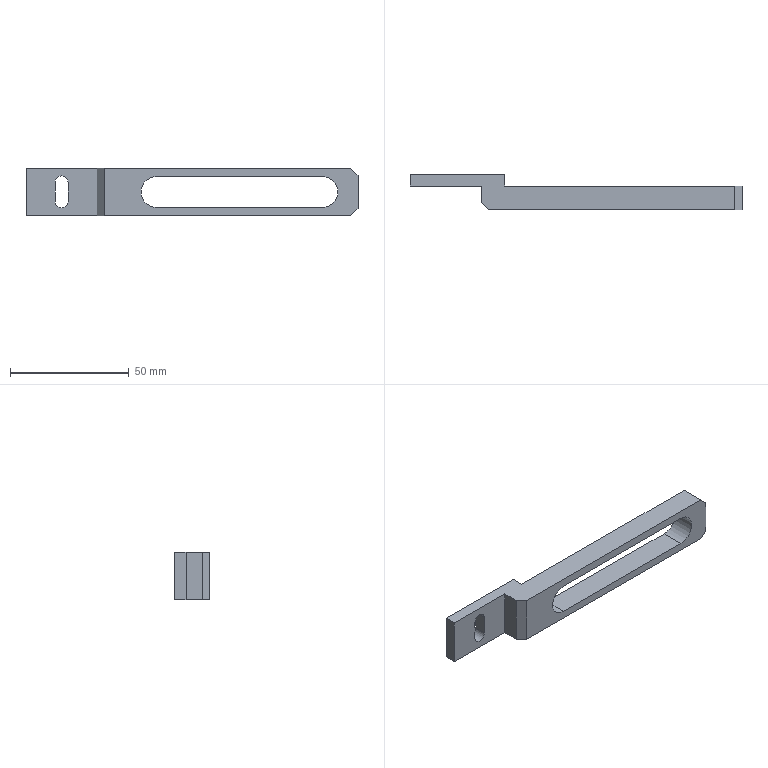Part | SolidWorks | features ICE 3, Chamfer 2, Extrusion 1 | 1 solid | 22 faces | box 140 x 15 x 20 mm | volume 15054 mm3 | plane 17 | cylinder 5 | commonest cylinder face diameters 5.5 x3 13 x2
STEP:
#1=CARTESIAN_POINT('',(15.,-5.,6.75));
#2=VERTEX_POINT('',#1);
#3=CARTESIAN_POINT('',(17.75,-5.,4.));
#4=VERTEX_POINT('',#3);
#5=CARTESIAN_POINT('',(15.,-5.,4.));
#6=DIRECTION('',(0.,1.,0.));
#7=DIRECTION('',(-1.,0.,0.));
#8=AXIS2_PLACEMENT_3D('',#5,#6,#7);
#9=CIRCLE('',#8,2.75);
#10=EDGE_CURVE('',#2,#4,#9,.T.);
#11=ORIENTED_EDGE('',*,*,#10,.F.);
#12=CARTESIAN_POINT('',(15.,0.,6.75));
#13=VERTEX_POINT('',#12);
#14=CARTESIAN_POINT('',(15.,-15.,6.75));
#15=DIRECTION('',(0.,1.,0.));
#16=VECTOR('',#15,1000.);
#17=LINE('',#14,#16);
#18=EDGE_CURVE('',#2,#13,#17,.T.);
#19=ORIENTED_EDGE('',*,*,#18,.T.);
#20=CARTESIAN_POINT('',(17.75,0.,4.));
#21=VERTEX_POINT('',#20);
#22=CARTESIAN_POINT('',(15.,0.,4.));
#23=DIRECTION('',(0.,1.,0.));
#24=DIRECTION('',(0.,0.,1.));
#25=AXIS2_PLACEMENT_3D('',#22,#23,#24);
#26=CIRCLE('',#25,2.75);
#27=EDGE_CURVE('',#13,#21,#26,.T.);
#28=ORIENTED_EDGE('',*,*,#27,.T.);
#29=CARTESIAN_POINT('',(17.75,-15.,4.));
#30=DIRECTION('',(0.,1.,0.));
#31=VECTOR('',#30,1000.);
#32=LINE('',#29,#31);
#33=EDGE_CURVE('',#4,#21,#32,.T.);
#34=ORIENTED_EDGE('',*,*,#33,.F.);
#35=EDGE_LOOP('',(#11,#19,#28,#34));
#36=FACE_OUTER_BOUND('',#35,.T.);
#37=CARTESIAN_POINT('',(15.,-15.,4.));
#38=DIRECTION('',(0.,1.,0.));
#39=DIRECTION('',(0.,0.,1.));
#40=AXIS2_PLACEMENT_3D('',#37,#38,#39);
#41=CYLINDRICAL_SURFACE('',#40,2.75);
#42=ADVANCED_FACE('',(#36),#41,.F.);
#43=CARTESIAN_POINT('',(0.,0.,-10.));
#44=VERTEX_POINT('',#43);
#45=CARTESIAN_POINT('',(0.,-5.,-10.));
#46=VERTEX_POINT('',#45);
#47=CARTESIAN_POINT('',(0.,-5.,-10.));
#48=DIRECTION('',(0.,-1.,0.));
#49=VECTOR('',#48,1000.);
#50=LINE('',#47,#49);
#51=EDGE_CURVE('',#44,#46,#50,.T.);
#52=ORIENTED_EDGE('',*,*,#51,.T.);
#53=CARTESIAN_POINT('',(0.,-5.,10.));
#54=VERTEX_POINT('',#53);
#55=CARTESIAN_POINT('',(0.,-5.,10.));
#56=DIRECTION('',(0.,0.,-1.));
#57=VECTOR('',#56,1000.);
#58=LINE('',#55,#57);
#59=EDGE_CURVE('',#54,#46,#58,.T.);
#60=ORIENTED_EDGE('',*,*,#59,.F.);
#61=CARTESIAN_POINT('',(0.,0.,10.));
#62=VERTEX_POINT('',#61);
#63=CARTESIAN_POINT('',(0.,-5.,10.));
#64=DIRECTION('',(0.,-1.,0.));
#65=VECTOR('',#64,1000.);
#66=LINE('',#63,#65);
#67=EDGE_CURVE('',#62,#54,#66,.T.);
#68=ORIENTED_EDGE('',*,*,#67,.F.);
#69=CARTESIAN_POINT('',(0.,0.,10.));
#70=DIRECTION('',(0.,0.,-1.));
#71=VECTOR('',#70,1000.);
#72=LINE('',#69,#71);
#73=EDGE_CURVE('',#62,#44,#72,.T.);
#74=ORIENTED_EDGE('',*,*,#73,.T.);
#75=EDGE_LOOP('',(#52,#60,#68,#74));
#76=FACE_OUTER_BOUND('',#75,.T.);
#77=CARTESIAN_POINT('',(0.,-5.,10.));
#78=DIRECTION('',(1.,0.,0.));
#79=DIRECTION('',(0.,0.,-1.));
#80=AXIS2_PLACEMENT_3D('',#77,#78,#79);
#81=PLANE('',#80);
#82=ADVANCED_FACE('',(#76),#81,.F.);
#83=CARTESIAN_POINT('',(17.75,-5.,-4.));
#84=VERTEX_POINT('',#83);
#85=CARTESIAN_POINT('',(17.75,-5.,10.));
#86=DIRECTION('',(0.,0.,-1.));
#87=VECTOR('',#86,1000.);
#88=LINE('',#85,#87);
#89=EDGE_CURVE('',#4,#84,#88,.T.);
#90=ORIENTED_EDGE('',*,*,#89,.T.);
#91=CARTESIAN_POINT('',(12.25,-5.,-4.));
#92=VERTEX_POINT('',#91);
#93=CARTESIAN_POINT('',(15.,-5.,-4.));
#94=DIRECTION('',(0.,1.,0.));
#95=DIRECTION('',(-1.,0.,0.));
#96=AXIS2_PLACEMENT_3D('',#93,#94,#95);
#97=CIRCLE('',#96,2.75);
#98=EDGE_CURVE('',#84,#92,#97,.T.);
#99=ORIENTED_EDGE('',*,*,#98,.T.);
#100=CARTESIAN_POINT('',(12.25,-5.,4.));
#101=VERTEX_POINT('',#100);
#102=CARTESIAN_POINT('',(12.25,-5.,10.));
#103=DIRECTION('',(0.,0.,1.));
#104=VECTOR('',#103,1000.);
#105=LINE('',#102,#104);
#106=EDGE_CURVE('',#92,#101,#105,.T.);
#107=ORIENTED_EDGE('',*,*,#106,.T.);
#108=CARTESIAN_POINT('',(15.,-5.,4.));
#109=DIRECTION('',(0.,1.,0.));
#110=DIRECTION('',(-1.,0.,0.));
#111=AXIS2_PLACEMENT_3D('',#108,#109,#110);
#112=CIRCLE('',#111,2.75);
#113=EDGE_CURVE('',#101,#2,#112,.T.);
#114=ORIENTED_EDGE('',*,*,#113,.T.);
#115=ORIENTED_EDGE('',*,*,#10,.T.);
#116=EDGE_LOOP('',(#90,#99,#107,#114,#115));
#117=FACE_BOUND('',#116,.T.);
#118=CARTESIAN_POINT('',(30.,-5.,-10.));
#119=VERTEX_POINT('',#118);
#120=CARTESIAN_POINT('',(30.,-5.,-10.));
#121=DIRECTION('',(1.,0.,0.));
#122=VECTOR('',#121,1000.);
#123=LINE('',#120,#122);
#124=EDGE_CURVE('',#46,#119,#123,.T.);
#125=ORIENTED_EDGE('',*,*,#124,.T.);
#126=CARTESIAN_POINT('',(30.,-5.,10.));
#127=VERTEX_POINT('',#126);
#128=CARTESIAN_POINT('',(30.,-5.,10.));
#129=DIRECTION('',(0.,0.,-1.));
#130=VECTOR('',#129,1000.);
#131=LINE('',#128,#130);
#132=EDGE_CURVE('',#127,#119,#131,.T.);
#133=ORIENTED_EDGE('',*,*,#132,.F.);
#134=CARTESIAN_POINT('',(30.,-5.,10.));
#135=DIRECTION('',(1.,0.,0.));
#136=VECTOR('',#135,1000.);
#137=LINE('',#134,#136);
#138=EDGE_CURVE('',#54,#127,#137,.T.);
#139=ORIENTED_EDGE('',*,*,#138,.F.);
#140=ORIENTED_EDGE('',*,*,#59,.T.);
#141=EDGE_LOOP('',(#125,#133,#139,#140));
#142=FACE_OUTER_BOUND('',#141,.T.);
#143=CARTESIAN_POINT('',(30.,-5.,10.));
#144=DIRECTION('',(0.,1.,0.));
#145=DIRECTION('',(-1.,0.,0.));
#146=AXIS2_PLACEMENT_3D('',#143,#144,#145);
#147=PLANE('',#146);
#148=ADVANCED_FACE('',(#117,#142),#147,.F.);
#149=CARTESIAN_POINT('',(30.,-12.,-10.));
#150=VERTEX_POINT('',#149);
#151=CARTESIAN_POINT('',(30.,-15.,-10.));
#152=DIRECTION('',(0.,-1.,0.));
#153=VECTOR('',#152,1000.);
#154=LINE('',#151,#153);
#155=EDGE_CURVE('',#119,#150,#154,.T.);
#156=ORIENTED_EDGE('',*,*,#155,.T.);
#157=CARTESIAN_POINT('',(30.,-12.,10.));
#158=VERTEX_POINT('',#157);
#159=CARTESIAN_POINT('',(30.,-12.,10.));
#160=DIRECTION('',(0.,0.,1.));
#161=VECTOR('',#160,1000.);
#162=LINE('',#159,#161);
#163=EDGE_CURVE('',#150,#158,#162,.T.);
#164=ORIENTED_EDGE('',*,*,#163,.T.);
#165=CARTESIAN_POINT('',(30.,-15.,10.));
#166=DIRECTION('',(0.,-1.,0.));
#167=VECTOR('',#166,1000.);
#168=LINE('',#165,#167);
#169=EDGE_CURVE('',#127,#158,#168,.T.);
#170=ORIENTED_EDGE('',*,*,#169,.F.);
#171=ORIENTED_EDGE('',*,*,#132,.T.);
#172=EDGE_LOOP('',(#156,#164,#170,#171));
#173=FACE_OUTER_BOUND('',#172,.T.);
#174=CARTESIAN_POINT('',(30.,-15.,10.));
#175=DIRECTION('',(1.,0.,0.));
#176=DIRECTION('',(0.,0.,-1.));
#177=AXIS2_PLACEMENT_3D('',#174,#175,#176);
#178=PLANE('',#177);
#179=ADVANCED_FACE('',(#173),#178,.F.);
#180=CARTESIAN_POINT('',(125.,-15.,-6.5));
#181=VERTEX_POINT('',#180);
#182=CARTESIAN_POINT('',(55.,-15.,-6.5));
#183=VERTEX_POINT('',#182);
#184=CARTESIAN_POINT('',(55.,-15.,-6.5));
#185=DIRECTION('',(-1.,0.,0.));
#186=VECTOR('',#185,1000.);
#187=LINE('',#184,#186);
#188=EDGE_CURVE('',#181,#183,#187,.T.);
#189=ORIENTED_EDGE('',*,*,#188,.T.);
#190=CARTESIAN_POINT('',(55.,-15.,6.5));
#191=VERTEX_POINT('',#190);
#192=CARTESIAN_POINT('',(55.,-15.,0.));
#193=DIRECTION('',(0.,1.,0.));
#194=DIRECTION('',(0.,0.,1.));
#195=AXIS2_PLACEMENT_3D('',#192,#193,#194);
#196=CIRCLE('',#195,6.5);
#197=EDGE_CURVE('',#183,#191,#196,.T.);
#198=ORIENTED_EDGE('',*,*,#197,.T.);
#199=CARTESIAN_POINT('',(125.,-15.,6.5));
#200=VERTEX_POINT('',#199);
#201=CARTESIAN_POINT('',(55.,-15.,6.5));
#202=DIRECTION('',(1.,0.,0.));
#203=VECTOR('',#202,1000.);
#204=LINE('',#201,#203);
#205=EDGE_CURVE('',#191,#200,#204,.T.);
#206=ORIENTED_EDGE('',*,*,#205,.T.);
#207=CARTESIAN_POINT('',(125.,-15.,0.));
#208=DIRECTION('',(0.,1.,0.));
#209=DIRECTION('',(0.,0.,1.));
#210=AXIS2_PLACEMENT_3D('',#207,#208,#209);
#211=CIRCLE('',#210,6.5);
#212=EDGE_CURVE('',#200,#181,#211,.T.);
#213=ORIENTED_EDGE('',*,*,#212,.T.);
#214=EDGE_LOOP('',(#189,#198,#206,#213));
#215=FACE_BOUND('',#214,.T.);
#216=CARTESIAN_POINT('',(33.,-15.,10.));
#217=VERTEX_POINT('',#216);
#218=CARTESIAN_POINT('',(137.,-15.,10.));
#219=VERTEX_POINT('',#218);
#220=CARTESIAN_POINT('',(140.,-15.,10.));
#221=DIRECTION('',(1.,0.,0.));
#222=VECTOR('',#221,1000.);
#223=LINE('',#220,#222);
#224=EDGE_CURVE('',#217,#219,#223,.T.);
#225=ORIENTED_EDGE('',*,*,#224,.F.);
#226=CARTESIAN_POINT('',(33.,-15.,-10.));
#227=VERTEX_POINT('',#226);
#228=CARTESIAN_POINT('',(33.,-15.,10.));
#229=DIRECTION('',(0.,0.,-1.));
#230=VECTOR('',#229,1000.);
#231=LINE('',#228,#230);
#232=EDGE_CURVE('',#217,#227,#231,.T.);
#233=ORIENTED_EDGE('',*,*,#232,.T.);
#234=CARTESIAN_POINT('',(137.,-15.,-10.));
#235=VERTEX_POINT('',#234);
#236=CARTESIAN_POINT('',(140.,-15.,-10.));
#237=DIRECTION('',(1.,0.,0.));
#238=VECTOR('',#237,1000.);
#239=LINE('',#236,#238);
#240=EDGE_CURVE('',#227,#235,#239,.T.);
#241=ORIENTED_EDGE('',*,*,#240,.T.);
#242=CARTESIAN_POINT('',(140.,-15.,-7.));
#243=VERTEX_POINT('',#242);
#244=CARTESIAN_POINT('',(140.,-15.,-7.));
#245=DIRECTION('',(0.7071,0.,0.7071));
#246=VECTOR('',#245,1000.);
#247=LINE('',#244,#246);
#248=EDGE_CURVE('',#235,#243,#247,.T.);
#249=ORIENTED_EDGE('',*,*,#248,.T.);
#250=CARTESIAN_POINT('',(140.,-15.,7.));
#251=VERTEX_POINT('',#250);
#252=CARTESIAN_POINT('',(140.,-15.,10.));
#253=DIRECTION('',(0.,0.,-1.));
#254=VECTOR('',#253,1000.);
#255=LINE('',#252,#254);
#256=EDGE_CURVE('',#251,#243,#255,.T.);
#257=ORIENTED_EDGE('',*,*,#256,.F.);
#258=CARTESIAN_POINT('',(137.,-15.,10.));
#259=DIRECTION('',(-0.7071,0.,0.7071));
#260=VECTOR('',#259,1000.);
#261=LINE('',#258,#260);
#262=EDGE_CURVE('',#251,#219,#261,.T.);
#263=ORIENTED_EDGE('',*,*,#262,.T.);
#264=EDGE_LOOP('',(#225,#233,#241,#249,#257,#263));
#265=FACE_OUTER_BOUND('',#264,.T.);
#266=CARTESIAN_POINT('',(140.,-15.,10.));
#267=DIRECTION('',(0.,1.,0.));
#268=DIRECTION('',(-1.,0.,0.));
#269=AXIS2_PLACEMENT_3D('',#266,#267,#268);
#270=PLANE('',#269);
#271=ADVANCED_FACE('',(#215,#265),#270,.F.);
#272=CARTESIAN_POINT('',(140.,-5.,-7.));
#273=VERTEX_POINT('',#272);
#274=CARTESIAN_POINT('',(140.,0.,-7.));
#275=DIRECTION('',(0.,1.,0.));
#276=VECTOR('',#275,1000.);
#277=LINE('',#274,#276);
#278=EDGE_CURVE('',#243,#273,#277,.T.);
#279=ORIENTED_EDGE('',*,*,#278,.T.);
#280=CARTESIAN_POINT('',(140.,-5.,7.));
#281=VERTEX_POINT('',#280);
#282=CARTESIAN_POINT('',(140.,-5.,-10.));
#283=DIRECTION('',(0.,0.,1.));
#284=VECTOR('',#283,1000.);
#285=LINE('',#282,#284);
#286=EDGE_CURVE('',#273,#281,#285,.T.);
#287=ORIENTED_EDGE('',*,*,#286,.T.);
#288=CARTESIAN_POINT('',(140.,0.,7.));
#289=DIRECTION('',(0.,-1.,0.));
#290=VECTOR('',#289,1000.);
#291=LINE('',#288,#290);
#292=EDGE_CURVE('',#281,#251,#291,.T.);
#293=ORIENTED_EDGE('',*,*,#292,.T.);
#294=ORIENTED_EDGE('',*,*,#256,.T.);
#295=EDGE_LOOP('',(#279,#287,#293,#294));
#296=FACE_OUTER_BOUND('',#295,.T.);
#297=CARTESIAN_POINT('',(140.,0.,10.));
#298=DIRECTION('',(-1.,0.,0.));
#299=DIRECTION('',(0.,0.,1.));
#300=AXIS2_PLACEMENT_3D('',#297,#298,#299);
#301=PLANE('',#300);
#302=ADVANCED_FACE('',(#296),#301,.F.);
#303=CARTESIAN_POINT('',(12.25,0.,-4.));
#304=VERTEX_POINT('',#303);
#305=CARTESIAN_POINT('',(12.25,0.,4.));
#306=VERTEX_POINT('',#305);
#307=CARTESIAN_POINT('',(12.25,0.,-4.));
#308=DIRECTION('',(0.,0.,1.));
#309=VECTOR('',#308,1000.);
#310=LINE('',#307,#309);
#311=EDGE_CURVE('',#304,#306,#310,.T.);
#312=ORIENTED_EDGE('',*,*,#311,.F.);
#313=CARTESIAN_POINT('',(17.75,0.,-4.));
#314=VERTEX_POINT('',#313);
#315=CARTESIAN_POINT('',(15.,0.,-4.));
#316=DIRECTION('',(0.,1.,0.));
#317=DIRECTION('',(0.,0.,1.));
#318=AXIS2_PLACEMENT_3D('',#315,#316,#317);
#319=CIRCLE('',#318,2.75);
#320=EDGE_CURVE('',#314,#304,#319,.T.);
#321=ORIENTED_EDGE('',*,*,#320,.F.);
#322=CARTESIAN_POINT('',(17.75,0.,-4.));
#323=DIRECTION('',(0.,0.,-1.));
#324=VECTOR('',#323,1000.);
#325=LINE('',#322,#324);
#326=EDGE_CURVE('',#21,#314,#325,.T.);
#327=ORIENTED_EDGE('',*,*,#326,.F.);
#328=ORIENTED_EDGE('',*,*,#27,.F.);
#329=CARTESIAN_POINT('',(15.,0.,4.));
#330=DIRECTION('',(0.,1.,0.));
#331=DIRECTION('',(0.,0.,1.));
#332=AXIS2_PLACEMENT_3D('',#329,#330,#331);
#333=CIRCLE('',#332,2.75);
#334=EDGE_CURVE('',#306,#13,#333,.T.);
#335=ORIENTED_EDGE('',*,*,#334,.F.);
#336=EDGE_LOOP('',(#312,#321,#327,#328,#335));
#337=FACE_BOUND('',#336,.T.);
#338=CARTESIAN_POINT('',(40.,0.,10.));
#339=VERTEX_POINT('',#338);
#340=CARTESIAN_POINT('',(0.,0.,10.));
#341=DIRECTION('',(-1.,0.,0.));
#342=VECTOR('',#341,1000.);
#343=LINE('',#340,#342);
#344=EDGE_CURVE('',#339,#62,#343,.T.);
#345=ORIENTED_EDGE('',*,*,#344,.F.);
#346=CARTESIAN_POINT('',(40.,0.,-10.));
#347=VERTEX_POINT('',#346);
#348=CARTESIAN_POINT('',(40.,0.,-10.));
#349=DIRECTION('',(0.,0.,1.));
#350=VECTOR('',#349,1000.);
#351=LINE('',#348,#350);
#352=EDGE_CURVE('',#347,#339,#351,.T.);
#353=ORIENTED_EDGE('',*,*,#352,.F.);
#354=CARTESIAN_POINT('',(0.,0.,-10.));
#355=DIRECTION('',(-1.,0.,0.));
#356=VECTOR('',#355,1000.);
#357=LINE('',#354,#356);
#358=EDGE_CURVE('',#347,#44,#357,.T.);
#359=ORIENTED_EDGE('',*,*,#358,.T.);
#360=ORIENTED_EDGE('',*,*,#73,.F.);
#361=EDGE_LOOP('',(#345,#353,#359,#360));
#362=FACE_OUTER_BOUND('',#361,.T.);
#363=CARTESIAN_POINT('',(0.,0.,10.));
#364=DIRECTION('',(0.,-1.,0.));
#365=DIRECTION('',(0.,0.,-1.));
#366=AXIS2_PLACEMENT_3D('',#363,#364,#365);
#367=PLANE('',#366);
#368=ADVANCED_FACE('',(#337,#362),#367,.F.);
#369=CARTESIAN_POINT('',(137.,-5.,10.));
#370=VERTEX_POINT('',#369);
#371=CARTESIAN_POINT('',(137.,0.,10.));
#372=DIRECTION('',(0.,1.,0.));
#373=VECTOR('',#372,1000.);
#374=LINE('',#371,#373);
#375=EDGE_CURVE('',#219,#370,#374,.T.);
#376=ORIENTED_EDGE('',*,*,#375,.T.);
#377=CARTESIAN_POINT('',(40.,-5.,10.));
#378=VERTEX_POINT('',#377);
#379=CARTESIAN_POINT('',(140.,-5.,10.));
#380=DIRECTION('',(1.,0.,0.));
#381=VECTOR('',#380,1000.);
#382=LINE('',#379,#381);
#383=EDGE_CURVE('',#378,#370,#382,.T.);
#384=ORIENTED_EDGE('',*,*,#383,.F.);
#385=CARTESIAN_POINT('',(40.,0.,10.));
#386=DIRECTION('',(0.,-1.,0.));
#387=VECTOR('',#386,1000.);
#388=LINE('',#385,#387);
#389=EDGE_CURVE('',#339,#378,#388,.T.);
#390=ORIENTED_EDGE('',*,*,#389,.F.);
#391=ORIENTED_EDGE('',*,*,#344,.T.);
#392=ORIENTED_EDGE('',*,*,#67,.T.);
#393=ORIENTED_EDGE('',*,*,#138,.T.);
#394=ORIENTED_EDGE('',*,*,#169,.T.);
#395=CARTESIAN_POINT('',(33.,-15.,10.));
#396=DIRECTION('',(0.7071,-0.7071,0.));
#397=VECTOR('',#396,1000.);
#398=LINE('',#395,#397);
#399=EDGE_CURVE('',#158,#217,#398,.T.);
#400=ORIENTED_EDGE('',*,*,#399,.T.);
#401=ORIENTED_EDGE('',*,*,#224,.T.);
#402=EDGE_LOOP('',(#376,#384,#390,#391,#392,#393,#394,#400,#401));
#403=FACE_OUTER_BOUND('',#402,.T.);
#404=CARTESIAN_POINT('',(0.,0.,10.));
#405=DIRECTION('',(0.,0.,-1.));
#406=DIRECTION('',(-1.,0.,0.));
#407=AXIS2_PLACEMENT_3D('',#404,#405,#406);
#408=PLANE('',#407);
#409=ADVANCED_FACE('',(#403),#408,.F.);
#410=CARTESIAN_POINT('',(40.,-5.,-10.));
#411=VERTEX_POINT('',#410);
#412=CARTESIAN_POINT('',(137.,-5.,-10.));
#413=VERTEX_POINT('',#412);
#414=CARTESIAN_POINT('',(140.,-5.,-10.));
#415=DIRECTION('',(1.,0.,0.));
#416=VECTOR('',#415,1000.);
#417=LINE('',#414,#416);
#418=EDGE_CURVE('',#411,#413,#417,.T.);
#419=ORIENTED_EDGE('',*,*,#418,.T.);
#420=CARTESIAN_POINT('',(137.,-15.,-10.));
#421=DIRECTION('',(0.,-1.,0.));
#422=VECTOR('',#421,1000.);
#423=LINE('',#420,#422);
#424=EDGE_CURVE('',#413,#235,#423,.T.);
#425=ORIENTED_EDGE('',*,*,#424,.T.);
#426=ORIENTED_EDGE('',*,*,#240,.F.);
#427=CARTESIAN_POINT('',(9.,9.,-10.));
#428=DIRECTION('',(-0.7071,0.7071,0.));
#429=VECTOR('',#428,1000.);
#430=LINE('',#427,#429);
#431=EDGE_CURVE('',#227,#150,#430,.T.);
#432=ORIENTED_EDGE('',*,*,#431,.T.);
#433=ORIENTED_EDGE('',*,*,#155,.F.);
#434=ORIENTED_EDGE('',*,*,#124,.F.);
#435=ORIENTED_EDGE('',*,*,#51,.F.);
#436=ORIENTED_EDGE('',*,*,#358,.F.);
#437=CARTESIAN_POINT('',(40.,0.,-10.));
#438=DIRECTION('',(0.,-1.,0.));
#439=VECTOR('',#438,1000.);
#440=LINE('',#437,#439);
#441=EDGE_CURVE('',#347,#411,#440,.T.);
#442=ORIENTED_EDGE('',*,*,#441,.T.);
#443=EDGE_LOOP('',(#419,#425,#426,#432,#433,#434,#435,#436,#442));
#444=FACE_OUTER_BOUND('',#443,.T.);
#445=CARTESIAN_POINT('',(0.,0.,-10.));
#446=DIRECTION('',(0.,0.,-1.));
#447=DIRECTION('',(-1.,0.,0.));
#448=AXIS2_PLACEMENT_3D('',#445,#446,#447);
#449=PLANE('',#448);
#450=ADVANCED_FACE('',(#444),#449,.T.);
#451=CARTESIAN_POINT('',(55.,-5.,-6.5));
#452=VERTEX_POINT('',#451);
#453=CARTESIAN_POINT('',(55.,-15.,-6.5));
#454=DIRECTION('',(0.,1.,0.));
#455=VECTOR('',#454,1000.);
#456=LINE('',#453,#455);
#457=EDGE_CURVE('',#183,#452,#456,.T.);
#458=ORIENTED_EDGE('',*,*,#457,.T.);
#459=CARTESIAN_POINT('',(55.,-5.,6.5));
#460=VERTEX_POINT('',#459);
#461=CARTESIAN_POINT('',(55.,-5.,0.));
#462=DIRECTION('',(0.,1.,0.));
#463=DIRECTION('',(1.,0.,0.));
#464=AXIS2_PLACEMENT_3D('',#461,#462,#463);
#465=CIRCLE('',#464,6.5);
#466=EDGE_CURVE('',#452,#460,#465,.T.);
#467=ORIENTED_EDGE('',*,*,#466,.T.);
#468=CARTESIAN_POINT('',(55.,-15.,6.5));
#469=DIRECTION('',(0.,1.,0.));
#470=VECTOR('',#469,1000.);
#471=LINE('',#468,#470);
#472=EDGE_CURVE('',#191,#460,#471,.T.);
#473=ORIENTED_EDGE('',*,*,#472,.F.);
#474=ORIENTED_EDGE('',*,*,#197,.F.);
#475=EDGE_LOOP('',(#458,#467,#473,#474));
#476=FACE_OUTER_BOUND('',#475,.T.);
#477=CARTESIAN_POINT('',(55.,-15.,0.));
#478=DIRECTION('',(0.,1.,0.));
#479=DIRECTION('',(0.,0.,1.));
#480=AXIS2_PLACEMENT_3D('',#477,#478,#479);
#481=CYLINDRICAL_SURFACE('',#480,6.5);
#482=ADVANCED_FACE('',(#476),#481,.F.);
#483=CARTESIAN_POINT('',(125.,-5.,-6.5));
#484=VERTEX_POINT('',#483);
#485=CARTESIAN_POINT('',(125.,-15.,-6.5));
#486=DIRECTION('',(0.,1.,0.));
#487=VECTOR('',#486,1000.);
#488=LINE('',#485,#487);
#489=EDGE_CURVE('',#181,#484,#488,.T.);
#490=ORIENTED_EDGE('',*,*,#489,.T.);
#491=CARTESIAN_POINT('',(55.,-5.,-6.5));
#492=DIRECTION('',(-1.,0.,0.));
#493=VECTOR('',#492,1000.);
#494=LINE('',#491,#493);
#495=EDGE_CURVE('',#484,#452,#494,.T.);
#496=ORIENTED_EDGE('',*,*,#495,.T.);
#497=ORIENTED_EDGE('',*,*,#457,.F.);
#498=ORIENTED_EDGE('',*,*,#188,.F.);
#499=EDGE_LOOP('',(#490,#496,#497,#498));
#500=FACE_OUTER_BOUND('',#499,.T.);
#501=CARTESIAN_POINT('',(55.,-15.,-6.5));
#502=DIRECTION('',(0.,0.,-1.));
#503=DIRECTION('',(-1.,0.,0.));
#504=AXIS2_PLACEMENT_3D('',#501,#502,#503);
#505=PLANE('',#504);
#506=ADVANCED_FACE('',(#500),#505,.F.);
#507=CARTESIAN_POINT('',(125.,-5.,6.5));
#508=VERTEX_POINT('',#507);
#509=CARTESIAN_POINT('',(125.,-15.,6.5));
#510=DIRECTION('',(0.,1.,0.));
#511=VECTOR('',#510,1000.);
#512=LINE('',#509,#511);
#513=EDGE_CURVE('',#200,#508,#512,.T.);
#514=ORIENTED_EDGE('',*,*,#513,.T.);
#515=CARTESIAN_POINT('',(125.,-5.,0.));
#516=DIRECTION('',(0.,1.,0.));
#517=DIRECTION('',(1.,0.,0.));
#518=AXIS2_PLACEMENT_3D('',#515,#516,#517);
#519=CIRCLE('',#518,6.5);
#520=EDGE_CURVE('',#508,#484,#519,.T.);
#521=ORIENTED_EDGE('',*,*,#520,.T.);
#522=ORIENTED_EDGE('',*,*,#489,.F.);
#523=ORIENTED_EDGE('',*,*,#212,.F.);
#524=EDGE_LOOP('',(#514,#521,#522,#523));
#525=FACE_OUTER_BOUND('',#524,.T.);
#526=CARTESIAN_POINT('',(125.,-15.,0.));
#527=DIRECTION('',(0.,1.,0.));
#528=DIRECTION('',(0.,0.,1.));
#529=AXIS2_PLACEMENT_3D('',#526,#527,#528);
#530=CYLINDRICAL_SURFACE('',#529,6.5);
#531=ADVANCED_FACE('',(#525),#530,.F.);
#532=ORIENTED_EDGE('',*,*,#472,.T.);
#533=CARTESIAN_POINT('',(55.,-5.,6.5));
#534=DIRECTION('',(1.,0.,0.));
#535=VECTOR('',#534,1000.);
#536=LINE('',#533,#535);
#537=EDGE_CURVE('',#460,#508,#536,.T.);
#538=ORIENTED_EDGE('',*,*,#537,.T.);
#539=ORIENTED_EDGE('',*,*,#513,.F.);
#540=ORIENTED_EDGE('',*,*,#205,.F.);
#541=EDGE_LOOP('',(#532,#538,#539,#540));
#542=FACE_OUTER_BOUND('',#541,.T.);
#543=CARTESIAN_POINT('',(55.,-15.,6.5));
#544=DIRECTION('',(0.,0.,1.));
#545=DIRECTION('',(1.,0.,0.));
#546=AXIS2_PLACEMENT_3D('',#543,#544,#545);
#547=PLANE('',#546);
#548=ADVANCED_FACE('',(#542),#547,.F.);
#549=CARTESIAN_POINT('',(17.75,-15.,-4.));
#550=DIRECTION('',(0.,1.,0.));
#551=VECTOR('',#550,1000.);
#552=LINE('',#549,#551);
#553=EDGE_CURVE('',#84,#314,#552,.T.);
#554=ORIENTED_EDGE('',*,*,#553,.T.);
#555=ORIENTED_EDGE('',*,*,#320,.T.);
#556=CARTESIAN_POINT('',(12.25,-15.,-4.));
#557=DIRECTION('',(0.,1.,0.));
#558=VECTOR('',#557,1000.);
#559=LINE('',#556,#558);
#560=EDGE_CURVE('',#92,#304,#559,.T.);
#561=ORIENTED_EDGE('',*,*,#560,.F.);
#562=ORIENTED_EDGE('',*,*,#98,.F.);
#563=EDGE_LOOP('',(#554,#555,#561,#562));
#564=FACE_OUTER_BOUND('',#563,.T.);
#565=CARTESIAN_POINT('',(15.,-15.,-4.));
#566=DIRECTION('',(0.,1.,0.));
#567=DIRECTION('',(0.,0.,1.));
#568=AXIS2_PLACEMENT_3D('',#565,#566,#567);
#569=CYLINDRICAL_SURFACE('',#568,2.75);
#570=ADVANCED_FACE('',(#564),#569,.F.);
#571=ORIENTED_EDGE('',*,*,#33,.T.);
#572=ORIENTED_EDGE('',*,*,#326,.T.);
#573=ORIENTED_EDGE('',*,*,#553,.F.);
#574=ORIENTED_EDGE('',*,*,#89,.F.);
#575=EDGE_LOOP('',(#571,#572,#573,#574));
#576=FACE_OUTER_BOUND('',#575,.T.);
#577=CARTESIAN_POINT('',(17.75,-15.,-4.));
#578=DIRECTION('',(1.,0.,0.));
#579=DIRECTION('',(0.,0.,-1.));
#580=AXIS2_PLACEMENT_3D('',#577,#578,#579);
#581=PLANE('',#580);
#582=ADVANCED_FACE('',(#576),#581,.F.);
#583=ORIENTED_EDGE('',*,*,#18,.F.);
#584=ORIENTED_EDGE('',*,*,#113,.F.);
#585=CARTESIAN_POINT('',(12.25,-15.,4.));
#586=DIRECTION('',(0.,1.,0.));
#587=VECTOR('',#586,1000.);
#588=LINE('',#585,#587);
#589=EDGE_CURVE('',#101,#306,#588,.T.);
#590=ORIENTED_EDGE('',*,*,#589,.T.);
#591=ORIENTED_EDGE('',*,*,#334,.T.);
#592=EDGE_LOOP('',(#583,#584,#590,#591));
#593=FACE_OUTER_BOUND('',#592,.T.);
#594=CARTESIAN_POINT('',(15.,-15.,4.));
#595=DIRECTION('',(0.,1.,0.));
#596=DIRECTION('',(0.,0.,1.));
#597=AXIS2_PLACEMENT_3D('',#594,#595,#596);
#598=CYLINDRICAL_SURFACE('',#597,2.75);
#599=ADVANCED_FACE('',(#593),#598,.F.);
#600=ORIENTED_EDGE('',*,*,#560,.T.);
#601=ORIENTED_EDGE('',*,*,#311,.T.);
#602=ORIENTED_EDGE('',*,*,#589,.F.);
#603=ORIENTED_EDGE('',*,*,#106,.F.);
#604=EDGE_LOOP('',(#600,#601,#602,#603));
#605=FACE_OUTER_BOUND('',#604,.T.);
#606=CARTESIAN_POINT('',(12.25,-15.,-4.));
#607=DIRECTION('',(-1.,0.,0.));
#608=DIRECTION('',(0.,0.,1.));
#609=AXIS2_PLACEMENT_3D('',#606,#607,#608);
#610=PLANE('',#609);
#611=ADVANCED_FACE('',(#605),#610,.F.);
#612=CARTESIAN_POINT('',(140.,-5.,-7.));
#613=DIRECTION('',(-0.7071,0.,-0.7071));
#614=VECTOR('',#613,1000.);
#615=LINE('',#612,#614);
#616=EDGE_CURVE('',#273,#413,#615,.T.);
#617=ORIENTED_EDGE('',*,*,#616,.F.);
#618=ORIENTED_EDGE('',*,*,#278,.F.);
#619=ORIENTED_EDGE('',*,*,#248,.F.);
#620=ORIENTED_EDGE('',*,*,#424,.F.);
#621=EDGE_LOOP('',(#617,#618,#619,#620));
#622=FACE_OUTER_BOUND('',#621,.T.);
#623=CARTESIAN_POINT('',(140.,0.,-7.));
#624=DIRECTION('',(0.7071,0.,-0.7071));
#625=DIRECTION('',(0.,-1.,0.));
#626=AXIS2_PLACEMENT_3D('',#623,#624,#625);
#627=PLANE('',#626);
#628=ADVANCED_FACE('',(#622),#627,.T.);
#629=CARTESIAN_POINT('',(137.,-5.,10.));
#630=DIRECTION('',(0.7071,0.,-0.7071));
#631=VECTOR('',#630,1000.);
#632=LINE('',#629,#631);
#633=EDGE_CURVE('',#370,#281,#632,.T.);
#634=ORIENTED_EDGE('',*,*,#633,.F.);
#635=ORIENTED_EDGE('',*,*,#375,.F.);
#636=ORIENTED_EDGE('',*,*,#262,.F.);
#637=ORIENTED_EDGE('',*,*,#292,.F.);
#638=EDGE_LOOP('',(#634,#635,#636,#637));
#639=FACE_OUTER_BOUND('',#638,.T.);
#640=CARTESIAN_POINT('',(137.,0.,10.));
#641=DIRECTION('',(-0.7071,0.,-0.7071));
#642=DIRECTION('',(0.,1.,0.));
#643=AXIS2_PLACEMENT_3D('',#640,#641,#642);
#644=PLANE('',#643);
#645=ADVANCED_FACE('',(#639),#644,.F.);
#646=ORIENTED_EDGE('',*,*,#399,.F.);
#647=ORIENTED_EDGE('',*,*,#163,.F.);
#648=ORIENTED_EDGE('',*,*,#431,.F.);
#649=ORIENTED_EDGE('',*,*,#232,.F.);
#650=EDGE_LOOP('',(#646,#647,#648,#649));
#651=FACE_OUTER_BOUND('',#650,.T.);
#652=CARTESIAN_POINT('',(33.,-15.,10.));
#653=DIRECTION('',(0.7071,0.7071,0.));
#654=DIRECTION('',(0.,0.,-1.));
#655=AXIS2_PLACEMENT_3D('',#652,#653,#654);
#656=PLANE('',#655);
#657=ADVANCED_FACE('',(#651),#656,.F.);
#658=ORIENTED_EDGE('',*,*,#616,.T.);
#659=ORIENTED_EDGE('',*,*,#418,.F.);
#660=CARTESIAN_POINT('',(40.,-5.,-10.));
#661=DIRECTION('',(0.,0.,1.));
#662=VECTOR('',#661,1000.);
#663=LINE('',#660,#662);
#664=EDGE_CURVE('',#411,#378,#663,.T.);
#665=ORIENTED_EDGE('',*,*,#664,.T.);
#666=ORIENTED_EDGE('',*,*,#383,.T.);
#667=ORIENTED_EDGE('',*,*,#633,.T.);
#668=ORIENTED_EDGE('',*,*,#286,.F.);
#669=EDGE_LOOP('',(#658,#659,#665,#666,#667,#668));
#670=FACE_OUTER_BOUND('',#669,.T.);
#671=ORIENTED_EDGE('',*,*,#495,.F.);
#672=ORIENTED_EDGE('',*,*,#520,.F.);
#673=ORIENTED_EDGE('',*,*,#537,.F.);
#674=ORIENTED_EDGE('',*,*,#466,.F.);
#675=EDGE_LOOP('',(#671,#672,#673,#674));
#676=FACE_BOUND('',#675,.T.);
#677=CARTESIAN_POINT('',(140.,-5.,-10.));
#678=DIRECTION('',(0.,-1.,0.));
#679=DIRECTION('',(1.,0.,0.));
#680=AXIS2_PLACEMENT_3D('',#677,#678,#679);
#681=PLANE('',#680);
#682=ADVANCED_FACE('',(#670,#676),#681,.F.);
#683=ORIENTED_EDGE('',*,*,#389,.T.);
#684=ORIENTED_EDGE('',*,*,#664,.F.);
#685=ORIENTED_EDGE('',*,*,#441,.F.);
#686=ORIENTED_EDGE('',*,*,#352,.T.);
#687=EDGE_LOOP('',(#683,#684,#685,#686));
#688=FACE_OUTER_BOUND('',#687,.T.);
#689=CARTESIAN_POINT('',(40.,0.,-10.));
#690=DIRECTION('',(-1.,0.,0.));
#691=DIRECTION('',(0.,0.,1.));
#692=AXIS2_PLACEMENT_3D('',#689,#690,#691);
#693=PLANE('',#692);
#694=ADVANCED_FACE('',(#688),#693,.F.);
#695=CLOSED_SHELL('',(#42,#82,#148,#179,#271,#302,#368,#409,#450,#482,#506,#531,#548,#570,#582,#599,#611,#628,#645,#657,#682,#694));
#696=MANIFOLD_SOLID_BREP('',#695);
#697=CARTESIAN_POINT('',(0.,0.,0.));
#698=DIRECTION('',(0.,0.,1.));
#699=DIRECTION('',(1.,0.,0.));
#700=AXIS2_PLACEMENT_3D('',#697,#698,#699);
#701=(LENGTH_UNIT()NAMED_UNIT(*)SI_UNIT(.MILLI.,.METRE.));
#702=UNCERTAINTY_MEASURE_WITH_UNIT(LENGTH_MEASURE(0.00001),#701,'','');
#703=(NAMED_UNIT(*)PLANE_ANGLE_UNIT()SI_UNIT($,.RADIAN.));
#704=(NAMED_UNIT(*)SI_UNIT($,.STERADIAN.)SOLID_ANGLE_UNIT());
#705=(GEOMETRIC_REPRESENTATION_CONTEXT(3)GLOBAL_UNCERTAINTY_ASSIGNED_CONTEXT((#702))GLOBAL_UNIT_ASSIGNED_CONTEXT((#701,#703,#704))REPRESENTATION_CONTEXT('',''));
#706=ADVANCED_BREP_SHAPE_REPRESENTATION('',(#696,#700),#705);